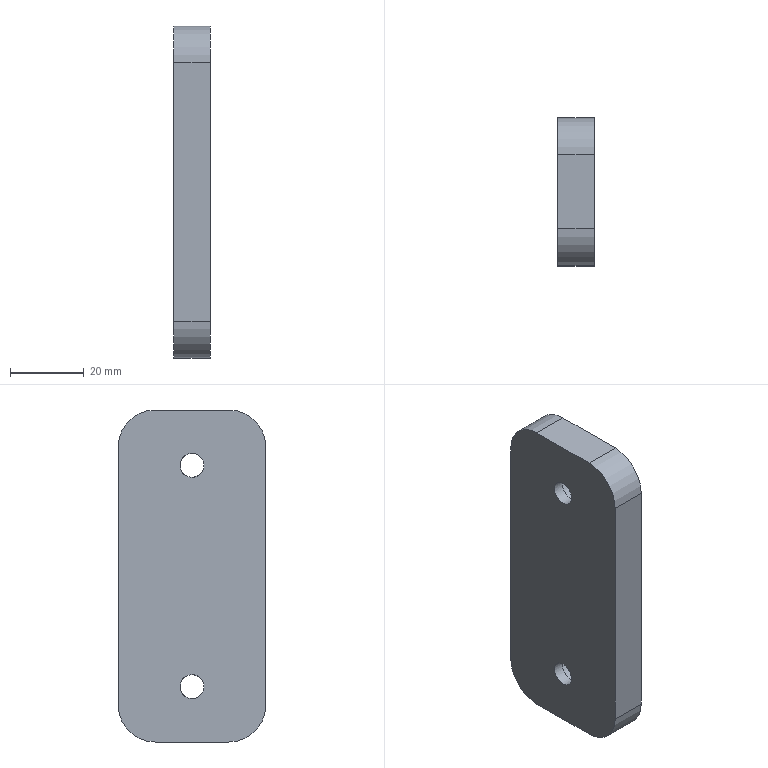Part | STEP file | solid 269 | 1 solid | 16 faces | box 10 x 40 x 90 mm | volume 33612 mm3 | plane 8 | cylinder 8 | commonest cylinder face diameters 20 x4 6.5 x2 11 x2